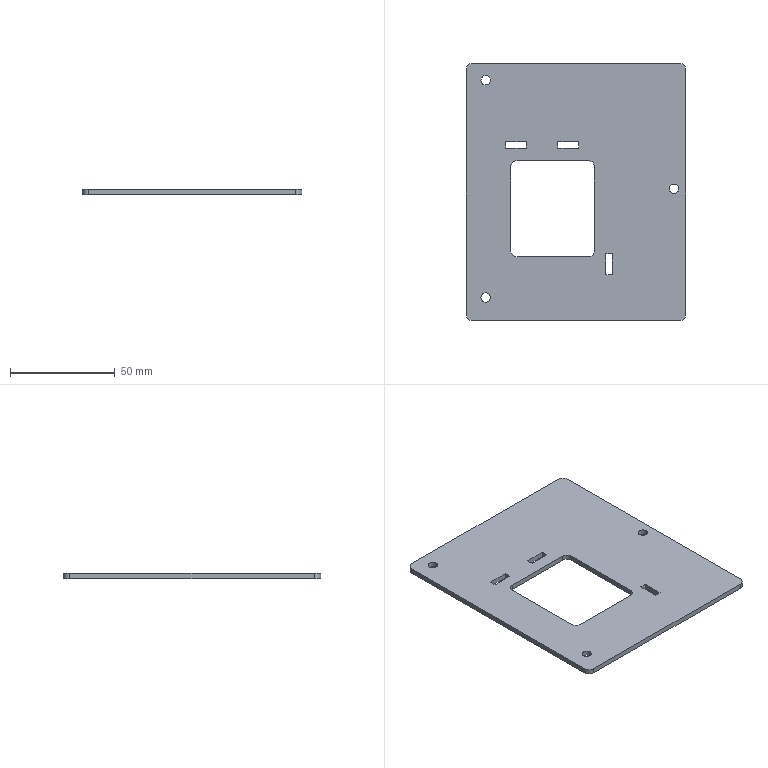Part | 1 solid | 36 faces | box 105 x 123 x 2.5 mm | volume 27343 mm3 | plane 22 | cylinder 14 | commonest cylinder face diameters 6 x8 4.5 x6
STEP:
#1=CARTESIAN_POINT('',(-45.448,-50.462,-2.5));
#2=VERTEX_POINT('',#1);
#3=CARTESIAN_POINT('',(-40.948,-50.462,-2.5));
#4=VERTEX_POINT('',#3);
#5=CARTESIAN_POINT('',(-43.198,-50.462,-2.5));
#6=DIRECTION('',(0.,0.,1.));
#7=DIRECTION('',(1.,0.,0.));
#8=AXIS2_PLACEMENT_3D('',#5,#6,#7);
#9=CIRCLE('',#8,2.25);
#10=EDGE_CURVE('',#2,#4,#9,.T.);
#11=ORIENTED_EDGE('',*,*,#10,.F.);
#12=CARTESIAN_POINT('',(-45.448,-50.462,0.));
#13=VERTEX_POINT('',#12);
#14=CARTESIAN_POINT('',(-45.448,-50.462,-10.));
#15=DIRECTION('',(0.,0.,1.));
#16=VECTOR('',#15,1000.);
#17=LINE('',#14,#16);
#18=EDGE_CURVE('',#2,#13,#17,.T.);
#19=ORIENTED_EDGE('',*,*,#18,.T.);
#20=CARTESIAN_POINT('',(-40.948,-50.462,0.));
#21=VERTEX_POINT('',#20);
#22=CARTESIAN_POINT('',(-43.198,-50.462,0.));
#23=DIRECTION('',(0.,0.,1.));
#24=DIRECTION('',(1.,0.,0.));
#25=AXIS2_PLACEMENT_3D('',#22,#23,#24);
#26=CIRCLE('',#25,2.25);
#27=EDGE_CURVE('',#13,#21,#26,.T.);
#28=ORIENTED_EDGE('',*,*,#27,.T.);
#29=CARTESIAN_POINT('',(-40.948,-50.462,-10.));
#30=DIRECTION('',(0.,0.,1.));
#31=VECTOR('',#30,1000.);
#32=LINE('',#29,#31);
#33=EDGE_CURVE('',#4,#21,#32,.T.);
#34=ORIENTED_EDGE('',*,*,#33,.F.);
#35=EDGE_LOOP('',(#11,#19,#28,#34));
#36=FACE_OUTER_BOUND('',#35,.T.);
#37=CARTESIAN_POINT('',(-43.198,-50.462,-10.));
#38=DIRECTION('',(0.,0.,1.));
#39=DIRECTION('',(1.,0.,0.));
#40=AXIS2_PLACEMENT_3D('',#37,#38,#39);
#41=CYLINDRICAL_SURFACE('',#40,2.25);
#42=ADVANCED_FACE('',(#36),#41,.F.);
#43=CARTESIAN_POINT('',(-45.448,53.462,-2.5));
#44=VERTEX_POINT('',#43);
#45=CARTESIAN_POINT('',(-40.948,53.462,-2.5));
#46=VERTEX_POINT('',#45);
#47=CARTESIAN_POINT('',(-43.198,53.462,-2.5));
#48=DIRECTION('',(0.,0.,1.));
#49=DIRECTION('',(1.,0.,0.));
#50=AXIS2_PLACEMENT_3D('',#47,#48,#49);
#51=CIRCLE('',#50,2.25);
#52=EDGE_CURVE('',#44,#46,#51,.T.);
#53=ORIENTED_EDGE('',*,*,#52,.F.);
#54=CARTESIAN_POINT('',(-45.448,53.462,0.));
#55=VERTEX_POINT('',#54);
#56=CARTESIAN_POINT('',(-45.448,53.462,-10.));
#57=DIRECTION('',(0.,0.,1.));
#58=VECTOR('',#57,1000.);
#59=LINE('',#56,#58);
#60=EDGE_CURVE('',#44,#55,#59,.T.);
#61=ORIENTED_EDGE('',*,*,#60,.T.);
#62=CARTESIAN_POINT('',(-40.948,53.462,0.));
#63=VERTEX_POINT('',#62);
#64=CARTESIAN_POINT('',(-43.198,53.462,0.));
#65=DIRECTION('',(0.,0.,1.));
#66=DIRECTION('',(1.,0.,0.));
#67=AXIS2_PLACEMENT_3D('',#64,#65,#66);
#68=CIRCLE('',#67,2.25);
#69=EDGE_CURVE('',#55,#63,#68,.T.);
#70=ORIENTED_EDGE('',*,*,#69,.T.);
#71=CARTESIAN_POINT('',(-40.948,53.462,-10.));
#72=DIRECTION('',(0.,0.,1.));
#73=VECTOR('',#72,1000.);
#74=LINE('',#71,#73);
#75=EDGE_CURVE('',#46,#63,#74,.T.);
#76=ORIENTED_EDGE('',*,*,#75,.F.);
#77=EDGE_LOOP('',(#53,#61,#70,#76));
#78=FACE_OUTER_BOUND('',#77,.T.);
#79=CARTESIAN_POINT('',(-43.198,53.462,-10.));
#80=DIRECTION('',(0.,0.,1.));
#81=DIRECTION('',(1.,0.,0.));
#82=AXIS2_PLACEMENT_3D('',#79,#80,#81);
#83=CYLINDRICAL_SURFACE('',#82,2.25);
#84=ADVANCED_FACE('',(#78),#83,.F.);
#85=CARTESIAN_POINT('',(44.552,1.5,-2.5));
#86=VERTEX_POINT('',#85);
#87=CARTESIAN_POINT('',(49.052,1.5,-2.5));
#88=VERTEX_POINT('',#87);
#89=CARTESIAN_POINT('',(46.802,1.5,-2.5));
#90=DIRECTION('',(0.,0.,1.));
#91=DIRECTION('',(1.,0.,0.));
#92=AXIS2_PLACEMENT_3D('',#89,#90,#91);
#93=CIRCLE('',#92,2.25);
#94=EDGE_CURVE('',#86,#88,#93,.T.);
#95=ORIENTED_EDGE('',*,*,#94,.F.);
#96=CARTESIAN_POINT('',(44.552,1.5,0.));
#97=VERTEX_POINT('',#96);
#98=CARTESIAN_POINT('',(44.552,1.5,-10.));
#99=DIRECTION('',(0.,0.,1.));
#100=VECTOR('',#99,1000.);
#101=LINE('',#98,#100);
#102=EDGE_CURVE('',#86,#97,#101,.T.);
#103=ORIENTED_EDGE('',*,*,#102,.T.);
#104=CARTESIAN_POINT('',(49.052,1.5,0.));
#105=VERTEX_POINT('',#104);
#106=CARTESIAN_POINT('',(46.802,1.5,0.));
#107=DIRECTION('',(0.,0.,1.));
#108=DIRECTION('',(1.,0.,0.));
#109=AXIS2_PLACEMENT_3D('',#106,#107,#108);
#110=CIRCLE('',#109,2.25);
#111=EDGE_CURVE('',#97,#105,#110,.T.);
#112=ORIENTED_EDGE('',*,*,#111,.T.);
#113=CARTESIAN_POINT('',(49.052,1.5,-10.));
#114=DIRECTION('',(0.,0.,1.));
#115=VECTOR('',#114,1000.);
#116=LINE('',#113,#115);
#117=EDGE_CURVE('',#88,#105,#116,.T.);
#118=ORIENTED_EDGE('',*,*,#117,.F.);
#119=EDGE_LOOP('',(#95,#103,#112,#118));
#120=FACE_OUTER_BOUND('',#119,.T.);
#121=CARTESIAN_POINT('',(46.802,1.5,-10.));
#122=DIRECTION('',(0.,0.,1.));
#123=DIRECTION('',(1.,0.,0.));
#124=AXIS2_PLACEMENT_3D('',#121,#122,#123);
#125=CYLINDRICAL_SURFACE('',#124,2.25);
#126=ADVANCED_FACE('',(#120),#125,.F.);
#127=CARTESIAN_POINT('',(52.5,-58.5,0.));
#128=VERTEX_POINT('',#127);
#129=CARTESIAN_POINT('',(52.5,58.5,0.));
#130=VERTEX_POINT('',#129);
#131=CARTESIAN_POINT('',(52.5,61.5,0.));
#132=DIRECTION('',(0.,1.,0.));
#133=VECTOR('',#132,1000.);
#134=LINE('',#131,#133);
#135=EDGE_CURVE('',#128,#130,#134,.T.);
#136=ORIENTED_EDGE('',*,*,#135,.F.);
#137=CARTESIAN_POINT('',(52.5,-58.5,-2.5));
#138=VERTEX_POINT('',#137);
#139=CARTESIAN_POINT('',(52.5,-58.5,-2.5));
#140=DIRECTION('',(0.,0.,-1.));
#141=VECTOR('',#140,1000.);
#142=LINE('',#139,#141);
#143=EDGE_CURVE('',#128,#138,#142,.T.);
#144=ORIENTED_EDGE('',*,*,#143,.T.);
#145=CARTESIAN_POINT('',(52.5,58.5,-2.5));
#146=VERTEX_POINT('',#145);
#147=CARTESIAN_POINT('',(52.5,61.5,-2.5));
#148=DIRECTION('',(0.,1.,0.));
#149=VECTOR('',#148,1000.);
#150=LINE('',#147,#149);
#151=EDGE_CURVE('',#138,#146,#150,.T.);
#152=ORIENTED_EDGE('',*,*,#151,.T.);
#153=CARTESIAN_POINT('',(52.5,58.5,-2.5));
#154=DIRECTION('',(0.,0.,1.));
#155=VECTOR('',#154,1000.);
#156=LINE('',#153,#155);
#157=EDGE_CURVE('',#146,#130,#156,.T.);
#158=ORIENTED_EDGE('',*,*,#157,.T.);
#159=EDGE_LOOP('',(#136,#144,#152,#158));
#160=FACE_OUTER_BOUND('',#159,.T.);
#161=CARTESIAN_POINT('',(52.5,61.5,-2.5));
#162=DIRECTION('',(1.,0.,0.));
#163=DIRECTION('',(0.,1.,0.));
#164=AXIS2_PLACEMENT_3D('',#161,#162,#163);
#165=PLANE('',#164);
#166=ADVANCED_FACE('',(#160),#165,.T.);
#167=CARTESIAN_POINT('',(-49.5,-61.5,-2.5));
#168=VERTEX_POINT('',#167);
#169=CARTESIAN_POINT('',(49.5,-61.5,-2.5));
#170=VERTEX_POINT('',#169);
#171=CARTESIAN_POINT('',(-52.5,-61.5,-2.5));
#172=DIRECTION('',(1.,0.,0.));
#173=VECTOR('',#172,1000.);
#174=LINE('',#171,#173);
#175=EDGE_CURVE('',#168,#170,#174,.T.);
#176=ORIENTED_EDGE('',*,*,#175,.T.);
#177=CARTESIAN_POINT('',(49.5,-61.5,0.));
#178=VERTEX_POINT('',#177);
#179=CARTESIAN_POINT('',(49.5,-61.5,-2.5));
#180=DIRECTION('',(0.,0.,1.));
#181=VECTOR('',#180,1000.);
#182=LINE('',#179,#181);
#183=EDGE_CURVE('',#170,#178,#182,.T.);
#184=ORIENTED_EDGE('',*,*,#183,.T.);
#185=CARTESIAN_POINT('',(-49.5,-61.5,0.));
#186=VERTEX_POINT('',#185);
#187=CARTESIAN_POINT('',(-52.5,-61.5,0.));
#188=DIRECTION('',(1.,0.,0.));
#189=VECTOR('',#188,1000.);
#190=LINE('',#187,#189);
#191=EDGE_CURVE('',#186,#178,#190,.T.);
#192=ORIENTED_EDGE('',*,*,#191,.F.);
#193=CARTESIAN_POINT('',(-49.5,-61.5,-2.5));
#194=DIRECTION('',(0.,0.,-1.));
#195=VECTOR('',#194,1000.);
#196=LINE('',#193,#195);
#197=EDGE_CURVE('',#186,#168,#196,.T.);
#198=ORIENTED_EDGE('',*,*,#197,.T.);
#199=EDGE_LOOP('',(#176,#184,#192,#198));
#200=FACE_OUTER_BOUND('',#199,.T.);
#201=CARTESIAN_POINT('',(-52.5,-61.5,-2.5));
#202=DIRECTION('',(0.,-1.,0.));
#203=DIRECTION('',(0.,0.,-1.));
#204=AXIS2_PLACEMENT_3D('',#201,#202,#203);
#205=PLANE('',#204);
#206=ADVANCED_FACE('',(#200),#205,.T.);
#207=CARTESIAN_POINT('',(-52.5,58.5,-2.5));
#208=VERTEX_POINT('',#207);
#209=CARTESIAN_POINT('',(-52.5,-58.5,-2.5));
#210=VERTEX_POINT('',#209);
#211=CARTESIAN_POINT('',(-52.5,61.5,-2.5));
#212=DIRECTION('',(0.,-1.,0.));
#213=VECTOR('',#212,1000.);
#214=LINE('',#211,#213);
#215=EDGE_CURVE('',#208,#210,#214,.T.);
#216=ORIENTED_EDGE('',*,*,#215,.T.);
#217=CARTESIAN_POINT('',(-52.5,-58.5,0.));
#218=VERTEX_POINT('',#217);
#219=CARTESIAN_POINT('',(-52.5,-58.5,-2.5));
#220=DIRECTION('',(0.,0.,1.));
#221=VECTOR('',#220,1000.);
#222=LINE('',#219,#221);
#223=EDGE_CURVE('',#210,#218,#222,.T.);
#224=ORIENTED_EDGE('',*,*,#223,.T.);
#225=CARTESIAN_POINT('',(-52.5,58.5,0.));
#226=VERTEX_POINT('',#225);
#227=CARTESIAN_POINT('',(-52.5,61.5,0.));
#228=DIRECTION('',(0.,-1.,0.));
#229=VECTOR('',#228,1000.);
#230=LINE('',#227,#229);
#231=EDGE_CURVE('',#226,#218,#230,.T.);
#232=ORIENTED_EDGE('',*,*,#231,.F.);
#233=CARTESIAN_POINT('',(-52.5,58.5,-2.5));
#234=DIRECTION('',(0.,0.,-1.));
#235=VECTOR('',#234,1000.);
#236=LINE('',#233,#235);
#237=EDGE_CURVE('',#226,#208,#236,.T.);
#238=ORIENTED_EDGE('',*,*,#237,.T.);
#239=EDGE_LOOP('',(#216,#224,#232,#238));
#240=FACE_OUTER_BOUND('',#239,.T.);
#241=CARTESIAN_POINT('',(-52.5,61.5,-2.5));
#242=DIRECTION('',(-1.,0.,0.));
#243=DIRECTION('',(0.,-1.,0.));
#244=AXIS2_PLACEMENT_3D('',#241,#242,#243);
#245=PLANE('',#244);
#246=ADVANCED_FACE('',(#240),#245,.T.);
#247=CARTESIAN_POINT('',(49.5,61.5,0.));
#248=VERTEX_POINT('',#247);
#249=CARTESIAN_POINT('',(-49.5,61.5,0.));
#250=VERTEX_POINT('',#249);
#251=CARTESIAN_POINT('',(-52.5,61.5,0.));
#252=DIRECTION('',(-1.,0.,0.));
#253=VECTOR('',#252,1000.);
#254=LINE('',#251,#253);
#255=EDGE_CURVE('',#248,#250,#254,.T.);
#256=ORIENTED_EDGE('',*,*,#255,.F.);
#257=CARTESIAN_POINT('',(49.5,61.5,-2.5));
#258=VERTEX_POINT('',#257);
#259=CARTESIAN_POINT('',(49.5,61.5,-2.5));
#260=DIRECTION('',(0.,0.,-1.));
#261=VECTOR('',#260,1000.);
#262=LINE('',#259,#261);
#263=EDGE_CURVE('',#248,#258,#262,.T.);
#264=ORIENTED_EDGE('',*,*,#263,.T.);
#265=CARTESIAN_POINT('',(-49.5,61.5,-2.5));
#266=VERTEX_POINT('',#265);
#267=CARTESIAN_POINT('',(-52.5,61.5,-2.5));
#268=DIRECTION('',(-1.,0.,0.));
#269=VECTOR('',#268,1000.);
#270=LINE('',#267,#269);
#271=EDGE_CURVE('',#258,#266,#270,.T.);
#272=ORIENTED_EDGE('',*,*,#271,.T.);
#273=CARTESIAN_POINT('',(-49.5,61.5,-2.5));
#274=DIRECTION('',(0.,0.,1.));
#275=VECTOR('',#274,1000.);
#276=LINE('',#273,#275);
#277=EDGE_CURVE('',#266,#250,#276,.T.);
#278=ORIENTED_EDGE('',*,*,#277,.T.);
#279=EDGE_LOOP('',(#256,#264,#272,#278));
#280=FACE_OUTER_BOUND('',#279,.T.);
#281=CARTESIAN_POINT('',(-52.5,61.5,-2.5));
#282=DIRECTION('',(0.,1.,0.));
#283=DIRECTION('',(0.,0.,1.));
#284=AXIS2_PLACEMENT_3D('',#281,#282,#283);
#285=PLANE('',#284);
#286=ADVANCED_FACE('',(#280),#285,.T.);
#287=CARTESIAN_POINT('',(17.302,-29.5,-2.5));
#288=VERTEX_POINT('',#287);
#289=CARTESIAN_POINT('',(14.302,-29.5,-2.5));
#290=VERTEX_POINT('',#289);
#291=CARTESIAN_POINT('',(0.,-29.5,-2.5));
#292=DIRECTION('',(-1.,0.,0.));
#293=VECTOR('',#292,1000.);
#294=LINE('',#291,#293);
#295=EDGE_CURVE('',#288,#290,#294,.T.);
#296=ORIENTED_EDGE('',*,*,#295,.T.);
#297=CARTESIAN_POINT('',(14.302,-39.5,-2.5));
#298=VERTEX_POINT('',#297);
#299=CARTESIAN_POINT('',(14.302,0.,-2.5));
#300=DIRECTION('',(0.,-1.,0.));
#301=VECTOR('',#300,1000.);
#302=LINE('',#299,#301);
#303=EDGE_CURVE('',#290,#298,#302,.T.);
#304=ORIENTED_EDGE('',*,*,#303,.T.);
#305=CARTESIAN_POINT('',(17.302,-39.5,-2.5));
#306=VERTEX_POINT('',#305);
#307=CARTESIAN_POINT('',(0.,-39.5,-2.5));
#308=DIRECTION('',(1.,0.,0.));
#309=VECTOR('',#308,1000.);
#310=LINE('',#307,#309);
#311=EDGE_CURVE('',#298,#306,#310,.T.);
#312=ORIENTED_EDGE('',*,*,#311,.T.);
#313=CARTESIAN_POINT('',(17.302,0.,-2.5));
#314=DIRECTION('',(0.,1.,0.));
#315=VECTOR('',#314,1000.);
#316=LINE('',#313,#315);
#317=EDGE_CURVE('',#306,#288,#316,.T.);
#318=ORIENTED_EDGE('',*,*,#317,.T.);
#319=EDGE_LOOP('',(#296,#304,#312,#318));
#320=FACE_BOUND('',#319,.T.);
#321=CARTESIAN_POINT('',(-33.698,21.,-2.5));
#322=VERTEX_POINT('',#321);
#323=CARTESIAN_POINT('',(-23.698,21.,-2.5));
#324=VERTEX_POINT('',#323);
#325=CARTESIAN_POINT('',(0.,21.,-2.5));
#326=DIRECTION('',(1.,0.,0.));
#327=VECTOR('',#326,1000.);
#328=LINE('',#325,#327);
#329=EDGE_CURVE('',#322,#324,#328,.T.);
#330=ORIENTED_EDGE('',*,*,#329,.T.);
#331=CARTESIAN_POINT('',(-23.698,24.,-2.5));
#332=VERTEX_POINT('',#331);
#333=CARTESIAN_POINT('',(-23.698,0.,-2.5));
#334=DIRECTION('',(0.,1.,0.));
#335=VECTOR('',#334,1000.);
#336=LINE('',#333,#335);
#337=EDGE_CURVE('',#324,#332,#336,.T.);
#338=ORIENTED_EDGE('',*,*,#337,.T.);
#339=CARTESIAN_POINT('',(-33.698,24.,-2.5));
#340=VERTEX_POINT('',#339);
#341=CARTESIAN_POINT('',(0.,24.,-2.5));
#342=DIRECTION('',(-1.,0.,0.));
#343=VECTOR('',#342,1000.);
#344=LINE('',#341,#343);
#345=EDGE_CURVE('',#332,#340,#344,.T.);
#346=ORIENTED_EDGE('',*,*,#345,.T.);
#347=CARTESIAN_POINT('',(-33.698,0.,-2.5));
#348=DIRECTION('',(0.,-1.,0.));
#349=VECTOR('',#348,1000.);
#350=LINE('',#347,#349);
#351=EDGE_CURVE('',#340,#322,#350,.T.);
#352=ORIENTED_EDGE('',*,*,#351,.T.);
#353=EDGE_LOOP('',(#330,#338,#346,#352));
#354=FACE_BOUND('',#353,.T.);
#355=CARTESIAN_POINT('',(-8.698,21.,-2.5));
#356=VERTEX_POINT('',#355);
#357=CARTESIAN_POINT('',(1.302,21.,-2.5));
#358=VERTEX_POINT('',#357);
#359=CARTESIAN_POINT('',(0.,21.,-2.5));
#360=DIRECTION('',(1.,0.,0.));
#361=VECTOR('',#360,1000.);
#362=LINE('',#359,#361);
#363=EDGE_CURVE('',#356,#358,#362,.T.);
#364=ORIENTED_EDGE('',*,*,#363,.T.);
#365=CARTESIAN_POINT('',(1.302,24.,-2.5));
#366=VERTEX_POINT('',#365);
#367=CARTESIAN_POINT('',(1.302,0.,-2.5));
#368=DIRECTION('',(0.,1.,0.));
#369=VECTOR('',#368,1000.);
#370=LINE('',#367,#369);
#371=EDGE_CURVE('',#358,#366,#370,.T.);
#372=ORIENTED_EDGE('',*,*,#371,.T.);
#373=CARTESIAN_POINT('',(-8.698,24.,-2.5));
#374=VERTEX_POINT('',#373);
#375=CARTESIAN_POINT('',(0.,24.,-2.5));
#376=DIRECTION('',(-1.,0.,0.));
#377=VECTOR('',#376,1000.);
#378=LINE('',#375,#377);
#379=EDGE_CURVE('',#366,#374,#378,.T.);
#380=ORIENTED_EDGE('',*,*,#379,.T.);
#381=CARTESIAN_POINT('',(-8.698,0.,-2.5));
#382=DIRECTION('',(0.,-1.,0.));
#383=VECTOR('',#382,1000.);
#384=LINE('',#381,#383);
#385=EDGE_CURVE('',#374,#356,#384,.T.);
#386=ORIENTED_EDGE('',*,*,#385,.T.);
#387=EDGE_LOOP('',(#364,#372,#380,#386));
#388=FACE_BOUND('',#387,.T.);
#389=CARTESIAN_POINT('',(-31.198,12.,-2.5));
#390=VERTEX_POINT('',#389);
#391=CARTESIAN_POINT('',(-31.198,-28.,-2.5));
#392=VERTEX_POINT('',#391);
#393=CARTESIAN_POINT('',(-31.198,0.,-2.5));
#394=DIRECTION('',(0.,-1.,0.));
#395=VECTOR('',#394,1000.);
#396=LINE('',#393,#395);
#397=EDGE_CURVE('',#390,#392,#396,.T.);
#398=ORIENTED_EDGE('',*,*,#397,.T.);
#399=CARTESIAN_POINT('',(-28.198,-31.,-2.5));
#400=VERTEX_POINT('',#399);
#401=CARTESIAN_POINT('',(-28.198,-28.,-2.5));
#402=DIRECTION('',(0.,0.,1.));
#403=DIRECTION('',(1.,0.,0.));
#404=AXIS2_PLACEMENT_3D('',#401,#402,#403);
#405=CIRCLE('',#404,3.);
#406=EDGE_CURVE('',#392,#400,#405,.T.);
#407=ORIENTED_EDGE('',*,*,#406,.T.);
#408=CARTESIAN_POINT('',(5.802,-31.,-2.5));
#409=VERTEX_POINT('',#408);
#410=CARTESIAN_POINT('',(0.,-31.,-2.5));
#411=DIRECTION('',(1.,0.,0.));
#412=VECTOR('',#411,1000.);
#413=LINE('',#410,#412);
#414=EDGE_CURVE('',#400,#409,#413,.T.);
#415=ORIENTED_EDGE('',*,*,#414,.T.);
#416=CARTESIAN_POINT('',(8.802,-28.,-2.5));
#417=VERTEX_POINT('',#416);
#418=CARTESIAN_POINT('',(5.802,-28.,-2.5));
#419=DIRECTION('',(0.,0.,1.));
#420=DIRECTION('',(1.,0.,0.));
#421=AXIS2_PLACEMENT_3D('',#418,#419,#420);
#422=CIRCLE('',#421,3.);
#423=EDGE_CURVE('',#409,#417,#422,.T.);
#424=ORIENTED_EDGE('',*,*,#423,.T.);
#425=CARTESIAN_POINT('',(8.802,12.,-2.5));
#426=VERTEX_POINT('',#425);
#427=CARTESIAN_POINT('',(8.802,0.,-2.5));
#428=DIRECTION('',(0.,1.,0.));
#429=VECTOR('',#428,1000.);
#430=LINE('',#427,#429);
#431=EDGE_CURVE('',#417,#426,#430,.T.);
#432=ORIENTED_EDGE('',*,*,#431,.T.);
#433=CARTESIAN_POINT('',(5.802,15.,-2.5));
#434=VERTEX_POINT('',#433);
#435=CARTESIAN_POINT('',(5.802,12.,-2.5));
#436=DIRECTION('',(0.,0.,1.));
#437=DIRECTION('',(1.,0.,0.));
#438=AXIS2_PLACEMENT_3D('',#435,#436,#437);
#439=CIRCLE('',#438,3.);
#440=EDGE_CURVE('',#426,#434,#439,.T.);
#441=ORIENTED_EDGE('',*,*,#440,.T.);
#442=CARTESIAN_POINT('',(-28.198,15.,-2.5));
#443=VERTEX_POINT('',#442);
#444=CARTESIAN_POINT('',(0.,15.,-2.5));
#445=DIRECTION('',(-1.,0.,0.));
#446=VECTOR('',#445,1000.);
#447=LINE('',#444,#446);
#448=EDGE_CURVE('',#434,#443,#447,.T.);
#449=ORIENTED_EDGE('',*,*,#448,.T.);
#450=CARTESIAN_POINT('',(-28.198,12.,-2.5));
#451=DIRECTION('',(0.,0.,1.));
#452=DIRECTION('',(1.,0.,0.));
#453=AXIS2_PLACEMENT_3D('',#450,#451,#452);
#454=CIRCLE('',#453,3.);
#455=EDGE_CURVE('',#443,#390,#454,.T.);
#456=ORIENTED_EDGE('',*,*,#455,.T.);
#457=EDGE_LOOP('',(#398,#407,#415,#424,#432,#441,#449,#456));
#458=FACE_BOUND('',#457,.T.);
#459=CARTESIAN_POINT('',(-43.198,-50.462,-2.5));
#460=DIRECTION('',(0.,0.,1.));
#461=DIRECTION('',(1.,0.,0.));
#462=AXIS2_PLACEMENT_3D('',#459,#460,#461);
#463=CIRCLE('',#462,2.25);
#464=EDGE_CURVE('',#4,#2,#463,.T.);
#465=ORIENTED_EDGE('',*,*,#464,.T.);
#466=ORIENTED_EDGE('',*,*,#10,.T.);
#467=EDGE_LOOP('',(#465,#466));
#468=FACE_BOUND('',#467,.T.);
#469=CARTESIAN_POINT('',(-43.198,53.462,-2.5));
#470=DIRECTION('',(0.,0.,1.));
#471=DIRECTION('',(1.,0.,0.));
#472=AXIS2_PLACEMENT_3D('',#469,#470,#471);
#473=CIRCLE('',#472,2.25);
#474=EDGE_CURVE('',#46,#44,#473,.T.);
#475=ORIENTED_EDGE('',*,*,#474,.T.);
#476=ORIENTED_EDGE('',*,*,#52,.T.);
#477=EDGE_LOOP('',(#475,#476));
#478=FACE_BOUND('',#477,.T.);
#479=CARTESIAN_POINT('',(46.802,1.5,-2.5));
#480=DIRECTION('',(0.,0.,1.));
#481=DIRECTION('',(1.,0.,0.));
#482=AXIS2_PLACEMENT_3D('',#479,#480,#481);
#483=CIRCLE('',#482,2.25);
#484=EDGE_CURVE('',#88,#86,#483,.T.);
#485=ORIENTED_EDGE('',*,*,#484,.T.);
#486=ORIENTED_EDGE('',*,*,#94,.T.);
#487=EDGE_LOOP('',(#485,#486));
#488=FACE_BOUND('',#487,.T.);
#489=ORIENTED_EDGE('',*,*,#151,.F.);
#490=CARTESIAN_POINT('',(49.5,-58.5,-2.5));
#491=DIRECTION('',(0.,0.,-1.));
#492=DIRECTION('',(1.,0.,0.));
#493=AXIS2_PLACEMENT_3D('',#490,#491,#492);
#494=CIRCLE('',#493,3.);
#495=EDGE_CURVE('',#138,#170,#494,.T.);
#496=ORIENTED_EDGE('',*,*,#495,.T.);
#497=ORIENTED_EDGE('',*,*,#175,.F.);
#498=CARTESIAN_POINT('',(-49.5,-58.5,-2.5));
#499=DIRECTION('',(0.,0.,-1.));
#500=DIRECTION('',(1.,0.,0.));
#501=AXIS2_PLACEMENT_3D('',#498,#499,#500);
#502=CIRCLE('',#501,3.);
#503=EDGE_CURVE('',#168,#210,#502,.T.);
#504=ORIENTED_EDGE('',*,*,#503,.T.);
#505=ORIENTED_EDGE('',*,*,#215,.F.);
#506=CARTESIAN_POINT('',(-49.5,58.5,-2.5));
#507=DIRECTION('',(0.,0.,-1.));
#508=DIRECTION('',(1.,0.,0.));
#509=AXIS2_PLACEMENT_3D('',#506,#507,#508);
#510=CIRCLE('',#509,3.);
#511=EDGE_CURVE('',#208,#266,#510,.T.);
#512=ORIENTED_EDGE('',*,*,#511,.T.);
#513=ORIENTED_EDGE('',*,*,#271,.F.);
#514=CARTESIAN_POINT('',(49.5,58.5,-2.5));
#515=DIRECTION('',(0.,0.,-1.));
#516=DIRECTION('',(1.,0.,0.));
#517=AXIS2_PLACEMENT_3D('',#514,#515,#516);
#518=CIRCLE('',#517,3.);
#519=EDGE_CURVE('',#258,#146,#518,.T.);
#520=ORIENTED_EDGE('',*,*,#519,.T.);
#521=EDGE_LOOP('',(#489,#496,#497,#504,#505,#512,#513,#520));
#522=FACE_OUTER_BOUND('',#521,.T.);
#523=CARTESIAN_POINT('',(0.,0.,-2.5));
#524=DIRECTION('',(0.,0.,1.));
#525=DIRECTION('',(1.,0.,0.));
#526=AXIS2_PLACEMENT_3D('',#523,#524,#525);
#527=PLANE('',#526);
#528=ADVANCED_FACE('',(#320,#354,#388,#458,#468,#478,#488,#522),#527,.F.);
#529=CARTESIAN_POINT('',(14.302,-29.5,0.));
#530=VERTEX_POINT('',#529);
#531=CARTESIAN_POINT('',(14.302,-39.5,0.));
#532=VERTEX_POINT('',#531);
#533=CARTESIAN_POINT('',(14.302,-39.5,0.));
#534=DIRECTION('',(0.,-1.,0.));
#535=VECTOR('',#534,1000.);
#536=LINE('',#533,#535);
#537=EDGE_CURVE('',#530,#532,#536,.T.);
#538=ORIENTED_EDGE('',*,*,#537,.F.);
#539=CARTESIAN_POINT('',(17.302,-29.5,0.));
#540=VERTEX_POINT('',#539);
#541=CARTESIAN_POINT('',(14.302,-29.5,0.));
#542=DIRECTION('',(-1.,0.,0.));
#543=VECTOR('',#542,1000.);
#544=LINE('',#541,#543);
#545=EDGE_CURVE('',#540,#530,#544,.T.);
#546=ORIENTED_EDGE('',*,*,#545,.F.);
#547=CARTESIAN_POINT('',(17.302,-39.5,0.));
#548=VERTEX_POINT('',#547);
#549=CARTESIAN_POINT('',(17.302,-39.5,0.));
#550=DIRECTION('',(0.,1.,0.));
#551=VECTOR('',#550,1000.);
#552=LINE('',#549,#551);
#553=EDGE_CURVE('',#548,#540,#552,.T.);
#554=ORIENTED_EDGE('',*,*,#553,.F.);
#555=CARTESIAN_POINT('',(14.302,-39.5,0.));
#556=DIRECTION('',(1.,0.,0.));
#557=VECTOR('',#556,1000.);
#558=LINE('',#555,#557);
#559=EDGE_CURVE('',#532,#548,#558,.T.);
#560=ORIENTED_EDGE('',*,*,#559,.F.);
#561=EDGE_LOOP('',(#538,#546,#554,#560));
#562=FACE_BOUND('',#561,.T.);
#563=CARTESIAN_POINT('',(-23.698,21.,0.));
#564=VERTEX_POINT('',#563);
#565=CARTESIAN_POINT('',(-23.698,24.,0.));
#566=VERTEX_POINT('',#565);
#567=CARTESIAN_POINT('',(-23.698,24.,0.));
#568=DIRECTION('',(0.,1.,0.));
#569=VECTOR('',#568,1000.);
#570=LINE('',#567,#569);
#571=EDGE_CURVE('',#564,#566,#570,.T.);
#572=ORIENTED_EDGE('',*,*,#571,.F.);
#573=CARTESIAN_POINT('',(-33.698,21.,0.));
#574=VERTEX_POINT('',#573);
#575=CARTESIAN_POINT('',(-23.698,21.,0.));
#576=DIRECTION('',(1.,0.,0.));
#577=VECTOR('',#576,1000.);
#578=LINE('',#575,#577);
#579=EDGE_CURVE('',#574,#564,#578,.T.);
#580=ORIENTED_EDGE('',*,*,#579,.F.);
#581=CARTESIAN_POINT('',(-33.698,24.,0.));
#582=VERTEX_POINT('',#581);
#583=CARTESIAN_POINT('',(-33.698,24.,0.));
#584=DIRECTION('',(0.,-1.,0.));
#585=VECTOR('',#584,1000.);
#586=LINE('',#583,#585);
#587=EDGE_CURVE('',#582,#574,#586,.T.);
#588=ORIENTED_EDGE('',*,*,#587,.F.);
#589=CARTESIAN_POINT('',(-23.698,24.,0.));
#590=DIRECTION('',(-1.,0.,0.));
#591=VECTOR('',#590,1000.);
#592=LINE('',#589,#591);
#593=EDGE_CURVE('',#566,#582,#592,.T.);
#594=ORIENTED_EDGE('',*,*,#593,.F.);
#595=EDGE_LOOP('',(#572,#580,#588,#594));
#596=FACE_BOUND('',#595,.T.);
#597=CARTESIAN_POINT('',(1.302,21.,0.));
#598=VERTEX_POINT('',#597);
#599=CARTESIAN_POINT('',(1.302,24.,0.));
#600=VERTEX_POINT('',#599);
#601=CARTESIAN_POINT('',(1.302,24.,0.));
#602=DIRECTION('',(0.,1.,0.));
#603=VECTOR('',#602,1000.);
#604=LINE('',#601,#603);
#605=EDGE_CURVE('',#598,#600,#604,.T.);
#606=ORIENTED_EDGE('',*,*,#605,.F.);
#607=CARTESIAN_POINT('',(-8.698,21.,0.));
#608=VERTEX_POINT('',#607);
#609=CARTESIAN_POINT('',(1.302,21.,0.));
#610=DIRECTION('',(1.,0.,0.));
#611=VECTOR('',#610,1000.);
#612=LINE('',#609,#611);
#613=EDGE_CURVE('',#608,#598,#612,.T.);
#614=ORIENTED_EDGE('',*,*,#613,.F.);
#615=CARTESIAN_POINT('',(-8.698,24.,0.));
#616=VERTEX_POINT('',#615);
#617=CARTESIAN_POINT('',(-8.698,24.,0.));
#618=DIRECTION('',(0.,-1.,0.));
#619=VECTOR('',#618,1000.);
#620=LINE('',#617,#619);
#621=EDGE_CURVE('',#616,#608,#620,.T.);
#622=ORIENTED_EDGE('',*,*,#621,.F.);
#623=CARTESIAN_POINT('',(1.302,24.,0.));
#624=DIRECTION('',(-1.,0.,0.));
#625=VECTOR('',#624,1000.);
#626=LINE('',#623,#625);
#627=EDGE_CURVE('',#600,#616,#626,.T.);
#628=ORIENTED_EDGE('',*,*,#627,.F.);
#629=EDGE_LOOP('',(#606,#614,#622,#628));
#630=FACE_BOUND('',#629,.T.);
#631=CARTESIAN_POINT('',(8.802,-28.,0.));
#632=VERTEX_POINT('',#631);
#633=CARTESIAN_POINT('',(8.802,12.,0.));
#634=VERTEX_POINT('',#633);
#635=CARTESIAN_POINT('',(8.802,15.,0.));
#636=DIRECTION('',(0.,1.,0.));
#637=VECTOR('',#636,1000.);
#638=LINE('',#635,#637);
#639=EDGE_CURVE('',#632,#634,#638,.T.);
#640=ORIENTED_EDGE('',*,*,#639,.F.);
#641=CARTESIAN_POINT('',(5.802,-31.,0.));
#642=VERTEX_POINT('',#641);
#643=CARTESIAN_POINT('',(5.802,-28.,0.));
#644=DIRECTION('',(0.,0.,-1.));
#645=DIRECTION('',(1.,0.,0.));
#646=AXIS2_PLACEMENT_3D('',#643,#644,#645);
#647=CIRCLE('',#646,3.);
#648=EDGE_CURVE('',#632,#642,#647,.T.);
#649=ORIENTED_EDGE('',*,*,#648,.T.);
#650=CARTESIAN_POINT('',(-28.198,-31.,0.));
#651=VERTEX_POINT('',#650);
#652=CARTESIAN_POINT('',(8.802,-31.,0.));
#653=DIRECTION('',(1.,0.,0.));
#654=VECTOR('',#653,1000.);
#655=LINE('',#652,#654);
#656=EDGE_CURVE('',#651,#642,#655,.T.);
#657=ORIENTED_EDGE('',*,*,#656,.F.);
#658=CARTESIAN_POINT('',(-31.198,-28.,0.));
#659=VERTEX_POINT('',#658);
#660=CARTESIAN_POINT('',(-28.198,-28.,0.));
#661=DIRECTION('',(0.,0.,-1.));
#662=DIRECTION('',(1.,0.,0.));
#663=AXIS2_PLACEMENT_3D('',#660,#661,#662);
#664=CIRCLE('',#663,3.);
#665=EDGE_CURVE('',#651,#659,#664,.T.);
#666=ORIENTED_EDGE('',*,*,#665,.T.);
#667=CARTESIAN_POINT('',(-31.198,12.,0.));
#668=VERTEX_POINT('',#667);
#669=CARTESIAN_POINT('',(-31.198,15.,0.));
#670=DIRECTION('',(0.,-1.,0.));
#671=VECTOR('',#670,1000.);
#672=LINE('',#669,#671);
#673=EDGE_CURVE('',#668,#659,#672,.T.);
#674=ORIENTED_EDGE('',*,*,#673,.F.);
#675=CARTESIAN_POINT('',(-28.198,15.,0.));
#676=VERTEX_POINT('',#675);
#677=CARTESIAN_POINT('',(-28.198,12.,0.));
#678=DIRECTION('',(0.,0.,-1.));
#679=DIRECTION('',(1.,0.,0.));
#680=AXIS2_PLACEMENT_3D('',#677,#678,#679);
#681=CIRCLE('',#680,3.);
#682=EDGE_CURVE('',#668,#676,#681,.T.);
#683=ORIENTED_EDGE('',*,*,#682,.T.);
#684=CARTESIAN_POINT('',(5.802,15.,0.));
#685=VERTEX_POINT('',#684);
#686=CARTESIAN_POINT('',(8.802,15.,0.));
#687=DIRECTION('',(-1.,0.,0.));
#688=VECTOR('',#687,1000.);
#689=LINE('',#686,#688);
#690=EDGE_CURVE('',#685,#676,#689,.T.);
#691=ORIENTED_EDGE('',*,*,#690,.F.);
#692=CARTESIAN_POINT('',(5.802,12.,0.));
#693=DIRECTION('',(0.,0.,-1.));
#694=DIRECTION('',(1.,0.,0.));
#695=AXIS2_PLACEMENT_3D('',#692,#693,#694);
#696=CIRCLE('',#695,3.);
#697=EDGE_CURVE('',#685,#634,#696,.T.);
#698=ORIENTED_EDGE('',*,*,#697,.T.);
#699=EDGE_LOOP('',(#640,#649,#657,#666,#674,#683,#691,#698));
#700=FACE_BOUND('',#699,.T.);
#701=CARTESIAN_POINT('',(-43.198,-50.462,0.));
#702=DIRECTION('',(0.,0.,1.));
#703=DIRECTION('',(1.,0.,0.));
#704=AXIS2_PLACEMENT_3D('',#701,#702,#703);
#705=CIRCLE('',#704,2.25);
#706=EDGE_CURVE('',#21,#13,#705,.T.);
#707=ORIENTED_EDGE('',*,*,#706,.F.);
#708=ORIENTED_EDGE('',*,*,#27,.F.);
#709=EDGE_LOOP('',(#707,#708));
#710=FACE_BOUND('',#709,.T.);
#711=CARTESIAN_POINT('',(-43.198,53.462,0.));
#712=DIRECTION('',(0.,0.,1.));
#713=DIRECTION('',(1.,0.,0.));
#714=AXIS2_PLACEMENT_3D('',#711,#712,#713);
#715=CIRCLE('',#714,2.25);
#716=EDGE_CURVE('',#63,#55,#715,.T.);
#717=ORIENTED_EDGE('',*,*,#716,.F.);
#718=ORIENTED_EDGE('',*,*,#69,.F.);
#719=EDGE_LOOP('',(#717,#718));
#720=FACE_BOUND('',#719,.T.);
#721=CARTESIAN_POINT('',(46.802,1.5,0.));
#722=DIRECTION('',(0.,0.,1.));
#723=DIRECTION('',(1.,0.,0.));
#724=AXIS2_PLACEMENT_3D('',#721,#722,#723);
#725=CIRCLE('',#724,2.25);
#726=EDGE_CURVE('',#105,#97,#725,.T.);
#727=ORIENTED_EDGE('',*,*,#726,.F.);
#728=ORIENTED_EDGE('',*,*,#111,.F.);
#729=EDGE_LOOP('',(#727,#728));
#730=FACE_BOUND('',#729,.T.);
#731=ORIENTED_EDGE('',*,*,#191,.T.);
#732=CARTESIAN_POINT('',(49.5,-58.5,0.));
#733=DIRECTION('',(0.,0.,1.));
#734=DIRECTION('',(1.,0.,0.));
#735=AXIS2_PLACEMENT_3D('',#732,#733,#734);
#736=CIRCLE('',#735,3.);
#737=EDGE_CURVE('',#178,#128,#736,.T.);
#738=ORIENTED_EDGE('',*,*,#737,.T.);
#739=ORIENTED_EDGE('',*,*,#135,.T.);
#740=CARTESIAN_POINT('',(49.5,58.5,0.));
#741=DIRECTION('',(0.,0.,1.));
#742=DIRECTION('',(1.,0.,0.));
#743=AXIS2_PLACEMENT_3D('',#740,#741,#742);
#744=CIRCLE('',#743,3.);
#745=EDGE_CURVE('',#130,#248,#744,.T.);
#746=ORIENTED_EDGE('',*,*,#745,.T.);
#747=ORIENTED_EDGE('',*,*,#255,.T.);
#748=CARTESIAN_POINT('',(-49.5,58.5,0.));
#749=DIRECTION('',(0.,0.,1.));
#750=DIRECTION('',(1.,0.,0.));
#751=AXIS2_PLACEMENT_3D('',#748,#749,#750);
#752=CIRCLE('',#751,3.);
#753=EDGE_CURVE('',#250,#226,#752,.T.);
#754=ORIENTED_EDGE('',*,*,#753,.T.);
#755=ORIENTED_EDGE('',*,*,#231,.T.);
#756=CARTESIAN_POINT('',(-49.5,-58.5,0.));
#757=DIRECTION('',(0.,0.,1.));
#758=DIRECTION('',(1.,0.,0.));
#759=AXIS2_PLACEMENT_3D('',#756,#757,#758);
#760=CIRCLE('',#759,3.);
#761=EDGE_CURVE('',#218,#186,#760,.T.);
#762=ORIENTED_EDGE('',*,*,#761,.T.);
#763=EDGE_LOOP('',(#731,#738,#739,#746,#747,#754,#755,#762));
#764=FACE_OUTER_BOUND('',#763,.T.);
#765=CARTESIAN_POINT('',(0.,0.,0.));
#766=DIRECTION('',(0.,0.,1.));
#767=DIRECTION('',(1.,0.,0.));
#768=AXIS2_PLACEMENT_3D('',#765,#766,#767);
#769=PLANE('',#768);
#770=ADVANCED_FACE('',(#562,#596,#630,#700,#710,#720,#730,#764),#769,.T.);
#771=ORIENTED_EDGE('',*,*,#495,.F.);
#772=ORIENTED_EDGE('',*,*,#143,.F.);
#773=ORIENTED_EDGE('',*,*,#737,.F.);
#774=ORIENTED_EDGE('',*,*,#183,.F.);
#775=EDGE_LOOP('',(#771,#772,#773,#774));
#776=FACE_OUTER_BOUND('',#775,.T.);
#777=CARTESIAN_POINT('',(49.5,-58.5,-2.5));
#778=DIRECTION('',(0.,0.,1.));
#779=DIRECTION('',(1.,0.,0.));
#780=AXIS2_PLACEMENT_3D('',#777,#778,#779);
#781=CYLINDRICAL_SURFACE('',#780,3.);
#782=ADVANCED_FACE('',(#776),#781,.T.);
#783=ORIENTED_EDGE('',*,*,#519,.F.);
#784=ORIENTED_EDGE('',*,*,#263,.F.);
#785=ORIENTED_EDGE('',*,*,#745,.F.);
#786=ORIENTED_EDGE('',*,*,#157,.F.);
#787=EDGE_LOOP('',(#783,#784,#785,#786));
#788=FACE_OUTER_BOUND('',#787,.T.);
#789=CARTESIAN_POINT('',(49.5,58.5,-2.5));
#790=DIRECTION('',(0.,0.,1.));
#791=DIRECTION('',(1.,0.,0.));
#792=AXIS2_PLACEMENT_3D('',#789,#790,#791);
#793=CYLINDRICAL_SURFACE('',#792,3.);
#794=ADVANCED_FACE('',(#788),#793,.T.);
#795=ORIENTED_EDGE('',*,*,#503,.F.);
#796=ORIENTED_EDGE('',*,*,#197,.F.);
#797=ORIENTED_EDGE('',*,*,#761,.F.);
#798=ORIENTED_EDGE('',*,*,#223,.F.);
#799=EDGE_LOOP('',(#795,#796,#797,#798));
#800=FACE_OUTER_BOUND('',#799,.T.);
#801=CARTESIAN_POINT('',(-49.5,-58.5,-2.5));
#802=DIRECTION('',(0.,0.,1.));
#803=DIRECTION('',(1.,0.,0.));
#804=AXIS2_PLACEMENT_3D('',#801,#802,#803);
#805=CYLINDRICAL_SURFACE('',#804,3.);
#806=ADVANCED_FACE('',(#800),#805,.T.);
#807=ORIENTED_EDGE('',*,*,#511,.F.);
#808=ORIENTED_EDGE('',*,*,#237,.F.);
#809=ORIENTED_EDGE('',*,*,#753,.F.);
#810=ORIENTED_EDGE('',*,*,#277,.F.);
#811=EDGE_LOOP('',(#807,#808,#809,#810));
#812=FACE_OUTER_BOUND('',#811,.T.);
#813=CARTESIAN_POINT('',(-49.5,58.5,-2.5));
#814=DIRECTION('',(0.,0.,1.));
#815=DIRECTION('',(1.,0.,0.));
#816=AXIS2_PLACEMENT_3D('',#813,#814,#815);
#817=CYLINDRICAL_SURFACE('',#816,3.);
#818=ADVANCED_FACE('',(#812),#817,.T.);
#819=ORIENTED_EDGE('',*,*,#102,.F.);
#820=ORIENTED_EDGE('',*,*,#484,.F.);
#821=ORIENTED_EDGE('',*,*,#117,.T.);
#822=ORIENTED_EDGE('',*,*,#726,.T.);
#823=EDGE_LOOP('',(#819,#820,#821,#822));
#824=FACE_OUTER_BOUND('',#823,.T.);
#825=CARTESIAN_POINT('',(46.802,1.5,-10.));
#826=DIRECTION('',(0.,0.,1.));
#827=DIRECTION('',(1.,0.,0.));
#828=AXIS2_PLACEMENT_3D('',#825,#826,#827);
#829=CYLINDRICAL_SURFACE('',#828,2.25);
#830=ADVANCED_FACE('',(#824),#829,.F.);
#831=ORIENTED_EDGE('',*,*,#60,.F.);
#832=ORIENTED_EDGE('',*,*,#474,.F.);
#833=ORIENTED_EDGE('',*,*,#75,.T.);
#834=ORIENTED_EDGE('',*,*,#716,.T.);
#835=EDGE_LOOP('',(#831,#832,#833,#834));
#836=FACE_OUTER_BOUND('',#835,.T.);
#837=CARTESIAN_POINT('',(-43.198,53.462,-10.));
#838=DIRECTION('',(0.,0.,1.));
#839=DIRECTION('',(1.,0.,0.));
#840=AXIS2_PLACEMENT_3D('',#837,#838,#839);
#841=CYLINDRICAL_SURFACE('',#840,2.25);
#842=ADVANCED_FACE('',(#836),#841,.F.);
#843=ORIENTED_EDGE('',*,*,#18,.F.);
#844=ORIENTED_EDGE('',*,*,#464,.F.);
#845=ORIENTED_EDGE('',*,*,#33,.T.);
#846=ORIENTED_EDGE('',*,*,#706,.T.);
#847=EDGE_LOOP('',(#843,#844,#845,#846));
#848=FACE_OUTER_BOUND('',#847,.T.);
#849=CARTESIAN_POINT('',(-43.198,-50.462,-10.));
#850=DIRECTION('',(0.,0.,1.));
#851=DIRECTION('',(1.,0.,0.));
#852=AXIS2_PLACEMENT_3D('',#849,#850,#851);
#853=CYLINDRICAL_SURFACE('',#852,2.25);
#854=ADVANCED_FACE('',(#848),#853,.F.);
#855=ORIENTED_EDGE('',*,*,#431,.F.);
#856=CARTESIAN_POINT('',(8.802,-28.,0.));
#857=DIRECTION('',(0.,0.,1.));
#858=VECTOR('',#857,1000.);
#859=LINE('',#856,#858);
#860=EDGE_CURVE('',#417,#632,#859,.T.);
#861=ORIENTED_EDGE('',*,*,#860,.T.);
#862=ORIENTED_EDGE('',*,*,#639,.T.);
#863=CARTESIAN_POINT('',(8.802,12.,-2.5));
#864=DIRECTION('',(0.,0.,-1.));
#865=VECTOR('',#864,1000.);
#866=LINE('',#863,#865);
#867=EDGE_CURVE('',#634,#426,#866,.T.);
#868=ORIENTED_EDGE('',*,*,#867,.T.);
#869=EDGE_LOOP('',(#855,#861,#862,#868));
#870=FACE_OUTER_BOUND('',#869,.T.);
#871=CARTESIAN_POINT('',(8.802,15.,-10.));
#872=DIRECTION('',(1.,0.,0.));
#873=DIRECTION('',(0.,1.,0.));
#874=AXIS2_PLACEMENT_3D('',#871,#872,#873);
#875=PLANE('',#874);
#876=ADVANCED_FACE('',(#870),#875,.F.);
#877=ORIENTED_EDGE('',*,*,#414,.F.);
#878=CARTESIAN_POINT('',(-28.198,-31.,0.));
#879=DIRECTION('',(0.,0.,1.));
#880=VECTOR('',#879,1000.);
#881=LINE('',#878,#880);
#882=EDGE_CURVE('',#400,#651,#881,.T.);
#883=ORIENTED_EDGE('',*,*,#882,.T.);
#884=ORIENTED_EDGE('',*,*,#656,.T.);
#885=CARTESIAN_POINT('',(5.802,-31.,-2.5));
#886=DIRECTION('',(0.,0.,-1.));
#887=VECTOR('',#886,1000.);
#888=LINE('',#885,#887);
#889=EDGE_CURVE('',#642,#409,#888,.T.);
#890=ORIENTED_EDGE('',*,*,#889,.T.);
#891=EDGE_LOOP('',(#877,#883,#884,#890));
#892=FACE_OUTER_BOUND('',#891,.T.);
#893=CARTESIAN_POINT('',(8.802,-31.,-10.));
#894=DIRECTION('',(0.,-1.,0.));
#895=DIRECTION('',(1.,0.,0.));
#896=AXIS2_PLACEMENT_3D('',#893,#894,#895);
#897=PLANE('',#896);
#898=ADVANCED_FACE('',(#892),#897,.F.);
#899=ORIENTED_EDGE('',*,*,#673,.T.);
#900=CARTESIAN_POINT('',(-31.198,-28.,-2.5));
#901=DIRECTION('',(0.,0.,-1.));
#902=VECTOR('',#901,1000.);
#903=LINE('',#900,#902);
#904=EDGE_CURVE('',#659,#392,#903,.T.);
#905=ORIENTED_EDGE('',*,*,#904,.T.);
#906=ORIENTED_EDGE('',*,*,#397,.F.);
#907=CARTESIAN_POINT('',(-31.198,12.,0.));
#908=DIRECTION('',(0.,0.,1.));
#909=VECTOR('',#908,1000.);
#910=LINE('',#907,#909);
#911=EDGE_CURVE('',#390,#668,#910,.T.);
#912=ORIENTED_EDGE('',*,*,#911,.T.);
#913=EDGE_LOOP('',(#899,#905,#906,#912));
#914=FACE_OUTER_BOUND('',#913,.T.);
#915=CARTESIAN_POINT('',(-31.198,15.,-10.));
#916=DIRECTION('',(-1.,0.,0.));
#917=DIRECTION('',(0.,-1.,0.));
#918=AXIS2_PLACEMENT_3D('',#915,#916,#917);
#919=PLANE('',#918);
#920=ADVANCED_FACE('',(#914),#919,.F.);
#921=ORIENTED_EDGE('',*,*,#448,.F.);
#922=CARTESIAN_POINT('',(5.802,15.,0.));
#923=DIRECTION('',(0.,0.,1.));
#924=VECTOR('',#923,1000.);
#925=LINE('',#922,#924);
#926=EDGE_CURVE('',#434,#685,#925,.T.);
#927=ORIENTED_EDGE('',*,*,#926,.T.);
#928=ORIENTED_EDGE('',*,*,#690,.T.);
#929=CARTESIAN_POINT('',(-28.198,15.,-2.5));
#930=DIRECTION('',(0.,0.,-1.));
#931=VECTOR('',#930,1000.);
#932=LINE('',#929,#931);
#933=EDGE_CURVE('',#676,#443,#932,.T.);
#934=ORIENTED_EDGE('',*,*,#933,.T.);
#935=EDGE_LOOP('',(#921,#927,#928,#934));
#936=FACE_OUTER_BOUND('',#935,.T.);
#937=CARTESIAN_POINT('',(8.802,15.,-10.));
#938=DIRECTION('',(0.,1.,0.));
#939=DIRECTION('',(-1.,0.,0.));
#940=AXIS2_PLACEMENT_3D('',#937,#938,#939);
#941=PLANE('',#940);
#942=ADVANCED_FACE('',(#936),#941,.F.);
#943=CARTESIAN_POINT('',(1.302,21.,-10.));
#944=DIRECTION('',(0.,0.,1.));
#945=VECTOR('',#944,1000.);
#946=LINE('',#943,#945);
#947=EDGE_CURVE('',#358,#598,#946,.T.);
#948=ORIENTED_EDGE('',*,*,#947,.T.);
#949=ORIENTED_EDGE('',*,*,#605,.T.);
#950=CARTESIAN_POINT('',(1.302,24.,-10.));
#951=DIRECTION('',(0.,0.,1.));
#952=VECTOR('',#951,1000.);
#953=LINE('',#950,#952);
#954=EDGE_CURVE('',#366,#600,#953,.T.);
#955=ORIENTED_EDGE('',*,*,#954,.F.);
#956=ORIENTED_EDGE('',*,*,#371,.F.);
#957=EDGE_LOOP('',(#948,#949,#955,#956));
#958=FACE_OUTER_BOUND('',#957,.T.);
#959=CARTESIAN_POINT('',(1.302,24.,-10.));
#960=DIRECTION('',(1.,0.,0.));
#961=DIRECTION('',(0.,0.,-1.));
#962=AXIS2_PLACEMENT_3D('',#959,#960,#961);
#963=PLANE('',#962);
#964=ADVANCED_FACE('',(#958),#963,.F.);
#965=CARTESIAN_POINT('',(-8.698,21.,-10.));
#966=DIRECTION('',(0.,0.,1.));
#967=VECTOR('',#966,1000.);
#968=LINE('',#965,#967);
#969=EDGE_CURVE('',#356,#608,#968,.T.);
#970=ORIENTED_EDGE('',*,*,#969,.T.);
#971=ORIENTED_EDGE('',*,*,#613,.T.);
#972=ORIENTED_EDGE('',*,*,#947,.F.);
#973=ORIENTED_EDGE('',*,*,#363,.F.);
#974=EDGE_LOOP('',(#970,#971,#972,#973));
#975=FACE_OUTER_BOUND('',#974,.T.);
#976=CARTESIAN_POINT('',(1.302,21.,-10.));
#977=DIRECTION('',(0.,-1.,0.));
#978=DIRECTION('',(0.,0.,-1.));
#979=AXIS2_PLACEMENT_3D('',#976,#977,#978);
#980=PLANE('',#979);
#981=ADVANCED_FACE('',(#975),#980,.F.);
#982=CARTESIAN_POINT('',(-8.698,24.,-10.));
#983=DIRECTION('',(0.,0.,1.));
#984=VECTOR('',#983,1000.);
#985=LINE('',#982,#984);
#986=EDGE_CURVE('',#374,#616,#985,.T.);
#987=ORIENTED_EDGE('',*,*,#986,.T.);
#988=ORIENTED_EDGE('',*,*,#621,.T.);
#989=ORIENTED_EDGE('',*,*,#969,.F.);
#990=ORIENTED_EDGE('',*,*,#385,.F.);
#991=EDGE_LOOP('',(#987,#988,#989,#990));
#992=FACE_OUTER_BOUND('',#991,.T.);
#993=CARTESIAN_POINT('',(-8.698,24.,-10.));
#994=DIRECTION('',(-1.,0.,0.));
#995=DIRECTION('',(0.,0.,1.));
#996=AXIS2_PLACEMENT_3D('',#993,#994,#995);
#997=PLANE('',#996);
#998=ADVANCED_FACE('',(#992),#997,.F.);
#999=ORIENTED_EDGE('',*,*,#954,.T.);
#1000=ORIENTED_EDGE('',*,*,#627,.T.);
#1001=ORIENTED_EDGE('',*,*,#986,.F.);
#1002=ORIENTED_EDGE('',*,*,#379,.F.);
#1003=EDGE_LOOP('',(#999,#1000,#1001,#1002));
#1004=FACE_OUTER_BOUND('',#1003,.T.);
#1005=CARTESIAN_POINT('',(1.302,24.,-10.));
#1006=DIRECTION('',(0.,1.,0.));
#1007=DIRECTION('',(0.,0.,1.));
#1008=AXIS2_PLACEMENT_3D('',#1005,#1006,#1007);
#1009=PLANE('',#1008);
#1010=ADVANCED_FACE('',(#1004),#1009,.F.);
#1011=CARTESIAN_POINT('',(-23.698,21.,-10.));
#1012=DIRECTION('',(0.,0.,1.));
#1013=VECTOR('',#1012,1000.);
#1014=LINE('',#1011,#1013);
#1015=EDGE_CURVE('',#324,#564,#1014,.T.);
#1016=ORIENTED_EDGE('',*,*,#1015,.T.);
#1017=ORIENTED_EDGE('',*,*,#571,.T.);
#1018=CARTESIAN_POINT('',(-23.698,24.,-10.));
#1019=DIRECTION('',(0.,0.,1.));
#1020=VECTOR('',#1019,1000.);
#1021=LINE('',#1018,#1020);
#1022=EDGE_CURVE('',#332,#566,#1021,.T.);
#1023=ORIENTED_EDGE('',*,*,#1022,.F.);
#1024=ORIENTED_EDGE('',*,*,#337,.F.);
#1025=EDGE_LOOP('',(#1016,#1017,#1023,#1024));
#1026=FACE_OUTER_BOUND('',#1025,.T.);
#1027=CARTESIAN_POINT('',(-23.698,24.,-10.));
#1028=DIRECTION('',(1.,0.,0.));
#1029=DIRECTION('',(0.,0.,-1.));
#1030=AXIS2_PLACEMENT_3D('',#1027,#1028,#1029);
#1031=PLANE('',#1030);
#1032=ADVANCED_FACE('',(#1026),#1031,.F.);
#1033=CARTESIAN_POINT('',(-33.698,21.,-10.));
#1034=DIRECTION('',(0.,0.,1.));
#1035=VECTOR('',#1034,1000.);
#1036=LINE('',#1033,#1035);
#1037=EDGE_CURVE('',#322,#574,#1036,.T.);
#1038=ORIENTED_EDGE('',*,*,#1037,.T.);
#1039=ORIENTED_EDGE('',*,*,#579,.T.);
#1040=ORIENTED_EDGE('',*,*,#1015,.F.);
#1041=ORIENTED_EDGE('',*,*,#329,.F.);
#1042=EDGE_LOOP('',(#1038,#1039,#1040,#1041));
#1043=FACE_OUTER_BOUND('',#1042,.T.);
#1044=CARTESIAN_POINT('',(-23.698,21.,-10.));
#1045=DIRECTION('',(0.,-1.,0.));
#1046=DIRECTION('',(0.,0.,-1.));
#1047=AXIS2_PLACEMENT_3D('',#1044,#1045,#1046);
#1048=PLANE('',#1047);
#1049=ADVANCED_FACE('',(#1043),#1048,.F.);
#1050=CARTESIAN_POINT('',(-33.698,24.,-10.));
#1051=DIRECTION('',(0.,0.,1.));
#1052=VECTOR('',#1051,1000.);
#1053=LINE('',#1050,#1052);
#1054=EDGE_CURVE('',#340,#582,#1053,.T.);
#1055=ORIENTED_EDGE('',*,*,#1054,.T.);
#1056=ORIENTED_EDGE('',*,*,#587,.T.);
#1057=ORIENTED_EDGE('',*,*,#1037,.F.);
#1058=ORIENTED_EDGE('',*,*,#351,.F.);
#1059=EDGE_LOOP('',(#1055,#1056,#1057,#1058));
#1060=FACE_OUTER_BOUND('',#1059,.T.);
#1061=CARTESIAN_POINT('',(-33.698,24.,-10.));
#1062=DIRECTION('',(-1.,0.,0.));
#1063=DIRECTION('',(0.,0.,1.));
#1064=AXIS2_PLACEMENT_3D('',#1061,#1062,#1063);
#1065=PLANE('',#1064);
#1066=ADVANCED_FACE('',(#1060),#1065,.F.);
#1067=ORIENTED_EDGE('',*,*,#1022,.T.);
#1068=ORIENTED_EDGE('',*,*,#593,.T.);
#1069=ORIENTED_EDGE('',*,*,#1054,.F.);
#1070=ORIENTED_EDGE('',*,*,#345,.F.);
#1071=EDGE_LOOP('',(#1067,#1068,#1069,#1070));
#1072=FACE_OUTER_BOUND('',#1071,.T.);
#1073=CARTESIAN_POINT('',(-23.698,24.,-10.));
#1074=DIRECTION('',(0.,1.,0.));
#1075=DIRECTION('',(0.,0.,1.));
#1076=AXIS2_PLACEMENT_3D('',#1073,#1074,#1075);
#1077=PLANE('',#1076);
#1078=ADVANCED_FACE('',(#1072),#1077,.F.);
#1079=CARTESIAN_POINT('',(14.302,-29.5,-10.));
#1080=DIRECTION('',(0.,0.,1.));
#1081=VECTOR('',#1080,1000.);
#1082=LINE('',#1079,#1081);
#1083=EDGE_CURVE('',#290,#530,#1082,.T.);
#1084=ORIENTED_EDGE('',*,*,#1083,.T.);
#1085=ORIENTED_EDGE('',*,*,#537,.T.);
#1086=CARTESIAN_POINT('',(14.302,-39.5,-10.));
#1087=DIRECTION('',(0.,0.,1.));
#1088=VECTOR('',#1087,1000.);
#1089=LINE('',#1086,#1088);
#1090=EDGE_CURVE('',#298,#532,#1089,.T.);
#1091=ORIENTED_EDGE('',*,*,#1090,.F.);
#1092=ORIENTED_EDGE('',*,*,#303,.F.);
#1093=EDGE_LOOP('',(#1084,#1085,#1091,#1092));
#1094=FACE_OUTER_BOUND('',#1093,.T.);
#1095=CARTESIAN_POINT('',(14.302,-39.5,-10.));
#1096=DIRECTION('',(-1.,0.,0.));
#1097=DIRECTION('',(0.,0.,1.));
#1098=AXIS2_PLACEMENT_3D('',#1095,#1096,#1097);
#1099=PLANE('',#1098);
#1100=ADVANCED_FACE('',(#1094),#1099,.F.);
#1101=CARTESIAN_POINT('',(17.302,-29.5,-10.));
#1102=DIRECTION('',(0.,0.,1.));
#1103=VECTOR('',#1102,1000.);
#1104=LINE('',#1101,#1103);
#1105=EDGE_CURVE('',#288,#540,#1104,.T.);
#1106=ORIENTED_EDGE('',*,*,#1105,.T.);
#1107=ORIENTED_EDGE('',*,*,#545,.T.);
#1108=ORIENTED_EDGE('',*,*,#1083,.F.);
#1109=ORIENTED_EDGE('',*,*,#295,.F.);
#1110=EDGE_LOOP('',(#1106,#1107,#1108,#1109));
#1111=FACE_OUTER_BOUND('',#1110,.T.);
#1112=CARTESIAN_POINT('',(14.302,-29.5,-10.));
#1113=DIRECTION('',(0.,1.,0.));
#1114=DIRECTION('',(0.,0.,1.));
#1115=AXIS2_PLACEMENT_3D('',#1112,#1113,#1114);
#1116=PLANE('',#1115);
#1117=ADVANCED_FACE('',(#1111),#1116,.F.);
#1118=CARTESIAN_POINT('',(17.302,-39.5,-10.));
#1119=DIRECTION('',(0.,0.,1.));
#1120=VECTOR('',#1119,1000.);
#1121=LINE('',#1118,#1120);
#1122=EDGE_CURVE('',#306,#548,#1121,.T.);
#1123=ORIENTED_EDGE('',*,*,#1122,.T.);
#1124=ORIENTED_EDGE('',*,*,#553,.T.);
#1125=ORIENTED_EDGE('',*,*,#1105,.F.);
#1126=ORIENTED_EDGE('',*,*,#317,.F.);
#1127=EDGE_LOOP('',(#1123,#1124,#1125,#1126));
#1128=FACE_OUTER_BOUND('',#1127,.T.);
#1129=CARTESIAN_POINT('',(17.302,-39.5,-10.));
#1130=DIRECTION('',(1.,0.,0.));
#1131=DIRECTION('',(0.,0.,-1.));
#1132=AXIS2_PLACEMENT_3D('',#1129,#1130,#1131);
#1133=PLANE('',#1132);
#1134=ADVANCED_FACE('',(#1128),#1133,.F.);
#1135=ORIENTED_EDGE('',*,*,#1090,.T.);
#1136=ORIENTED_EDGE('',*,*,#559,.T.);
#1137=ORIENTED_EDGE('',*,*,#1122,.F.);
#1138=ORIENTED_EDGE('',*,*,#311,.F.);
#1139=EDGE_LOOP('',(#1135,#1136,#1137,#1138));
#1140=FACE_OUTER_BOUND('',#1139,.T.);
#1141=CARTESIAN_POINT('',(14.302,-39.5,-10.));
#1142=DIRECTION('',(0.,-1.,0.));
#1143=DIRECTION('',(0.,0.,-1.));
#1144=AXIS2_PLACEMENT_3D('',#1141,#1142,#1143);
#1145=PLANE('',#1144);
#1146=ADVANCED_FACE('',(#1140),#1145,.F.);
#1147=ORIENTED_EDGE('',*,*,#406,.F.);
#1148=ORIENTED_EDGE('',*,*,#904,.F.);
#1149=ORIENTED_EDGE('',*,*,#665,.F.);
#1150=ORIENTED_EDGE('',*,*,#882,.F.);
#1151=EDGE_LOOP('',(#1147,#1148,#1149,#1150));
#1152=FACE_OUTER_BOUND('',#1151,.T.);
#1153=CARTESIAN_POINT('',(-28.198,-28.,-10.));
#1154=DIRECTION('',(0.,0.,-1.));
#1155=DIRECTION('',(-1.,0.,0.));
#1156=AXIS2_PLACEMENT_3D('',#1153,#1154,#1155);
#1157=CYLINDRICAL_SURFACE('',#1156,3.);
#1158=ADVANCED_FACE('',(#1152),#1157,.F.);
#1159=ORIENTED_EDGE('',*,*,#423,.F.);
#1160=ORIENTED_EDGE('',*,*,#889,.F.);
#1161=ORIENTED_EDGE('',*,*,#648,.F.);
#1162=ORIENTED_EDGE('',*,*,#860,.F.);
#1163=EDGE_LOOP('',(#1159,#1160,#1161,#1162));
#1164=FACE_OUTER_BOUND('',#1163,.T.);
#1165=CARTESIAN_POINT('',(5.802,-28.,-10.));
#1166=DIRECTION('',(0.,0.,-1.));
#1167=DIRECTION('',(-1.,0.,0.));
#1168=AXIS2_PLACEMENT_3D('',#1165,#1166,#1167);
#1169=CYLINDRICAL_SURFACE('',#1168,3.);
#1170=ADVANCED_FACE('',(#1164),#1169,.F.);
#1171=ORIENTED_EDGE('',*,*,#440,.F.);
#1172=ORIENTED_EDGE('',*,*,#867,.F.);
#1173=ORIENTED_EDGE('',*,*,#697,.F.);
#1174=ORIENTED_EDGE('',*,*,#926,.F.);
#1175=EDGE_LOOP('',(#1171,#1172,#1173,#1174));
#1176=FACE_OUTER_BOUND('',#1175,.T.);
#1177=CARTESIAN_POINT('',(5.802,12.,-10.));
#1178=DIRECTION('',(0.,0.,-1.));
#1179=DIRECTION('',(-1.,0.,0.));
#1180=AXIS2_PLACEMENT_3D('',#1177,#1178,#1179);
#1181=CYLINDRICAL_SURFACE('',#1180,3.);
#1182=ADVANCED_FACE('',(#1176),#1181,.F.);
#1183=ORIENTED_EDGE('',*,*,#455,.F.);
#1184=ORIENTED_EDGE('',*,*,#933,.F.);
#1185=ORIENTED_EDGE('',*,*,#682,.F.);
#1186=ORIENTED_EDGE('',*,*,#911,.F.);
#1187=EDGE_LOOP('',(#1183,#1184,#1185,#1186));
#1188=FACE_OUTER_BOUND('',#1187,.T.);
#1189=CARTESIAN_POINT('',(-28.198,12.,-10.));
#1190=DIRECTION('',(0.,0.,-1.));
#1191=DIRECTION('',(-1.,0.,0.));
#1192=AXIS2_PLACEMENT_3D('',#1189,#1190,#1191);
#1193=CYLINDRICAL_SURFACE('',#1192,3.);
#1194=ADVANCED_FACE('',(#1188),#1193,.F.);
#1195=CLOSED_SHELL('',(#42,#84,#126,#166,#206,#246,#286,#528,#770,#782,#794,#806,#818,#830,#842,#854,#876,#898,#920,#942,#964,#981,#998,#1010,#1032,#1049,#1066,#1078,#1100,#1117,#1134,#1146,#1158,#1170,#1182,#1194));
#1196=MANIFOLD_SOLID_BREP('',#1195);
#1197=CARTESIAN_POINT('',(0.,0.,0.));
#1198=DIRECTION('',(0.,0.,1.));
#1199=DIRECTION('',(1.,0.,0.));
#1200=AXIS2_PLACEMENT_3D('',#1197,#1198,#1199);
#1201=(LENGTH_UNIT()NAMED_UNIT(*)SI_UNIT(.MILLI.,.METRE.));
#1202=UNCERTAINTY_MEASURE_WITH_UNIT(LENGTH_MEASURE(0.00001),#1201,'','');
#1203=(NAMED_UNIT(*)PLANE_ANGLE_UNIT()SI_UNIT($,.RADIAN.));
#1204=(NAMED_UNIT(*)SI_UNIT($,.STERADIAN.)SOLID_ANGLE_UNIT());
#1205=(GEOMETRIC_REPRESENTATION_CONTEXT(3)GLOBAL_UNCERTAINTY_ASSIGNED_CONTEXT((#1202))GLOBAL_UNIT_ASSIGNED_CONTEXT((#1201,#1203,#1204))REPRESENTATION_CONTEXT('',''));
#1206=ADVANCED_BREP_SHAPE_REPRESENTATION('',(#1196,#1200),#1205);